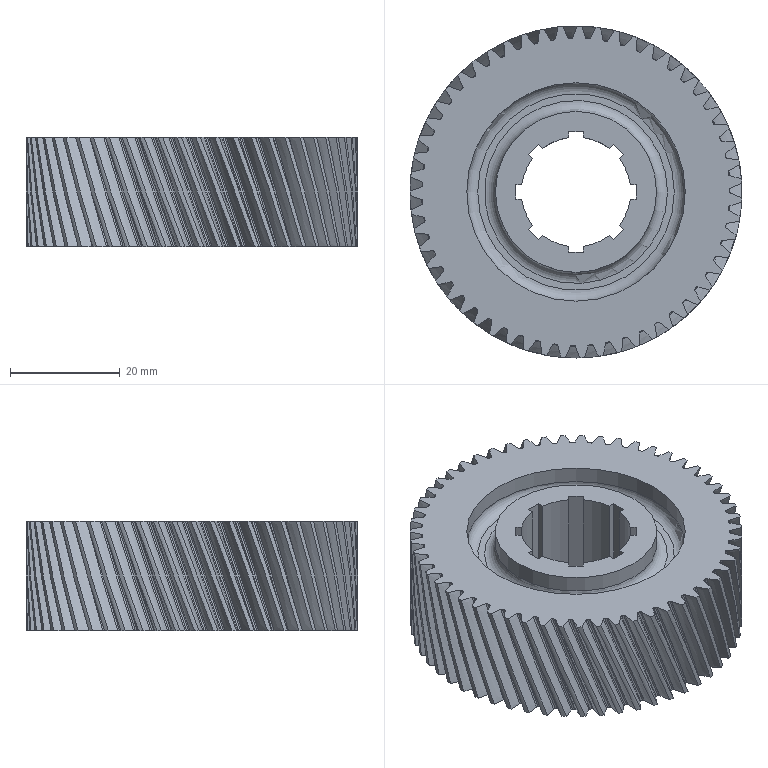Part | NX | features BREP 55, META 55, DATUM_CSYS 3, EXTRUDE 3, SKETCH 2, BLEND 1, CYLINDER 1, FSET 1 | 1 solid | 376 faces | volume 41545 mm3 | spline 275 | cylinder 67 | plane 30 | torus 4 | commonest cylinder face diameters 56.03 x55 20 x8 29.385 x2 39.836 x2